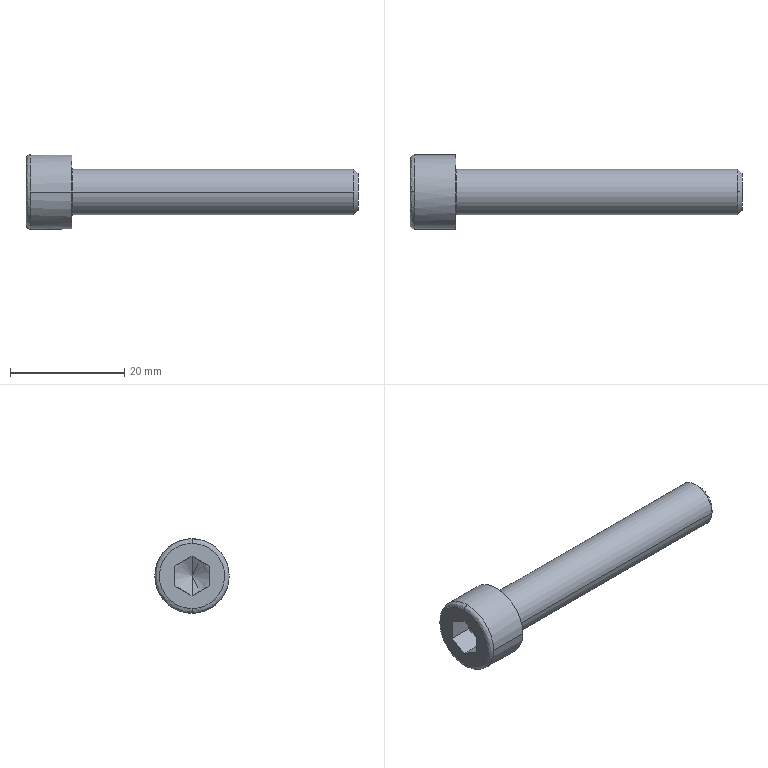Part | STEP file | DIN 912 - replaced by DIN EN ISO 4762 M8 x 50 | 1 solid | 21 faces | box 58 x 13 x 13 mm | volume 3414 mm3 | plane 9 | spline 4 | cylinder 4 | cone 4 | commonest cylinder face diameters 8 x2 13 x2